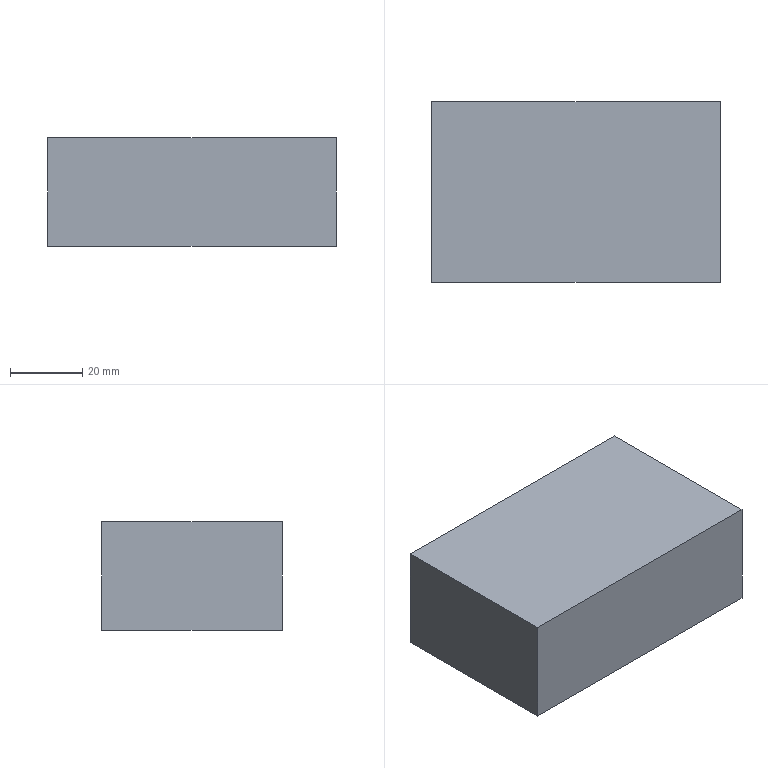Part | NX | features solid 2 | 1 solid | 6 faces | box 80 x 50 x 30 mm | volume 120000 mm3 | plane 6
STEP:
#1=CARTESIAN_POINT('',(41.,-178.,230.));
#2=VERTEX_POINT('',#1);
#3=CARTESIAN_POINT('',(41.,-128.,230.));
#4=VERTEX_POINT('',#3);
#5=CARTESIAN_POINT('',(41.,-467.676,230.));
#6=DIRECTION('',(0.,-1.,0.));
#7=VECTOR('',#6,1000.);
#8=LINE('',#5,#7);
#9=EDGE_CURVE('',#2,#4,#8,.F.);
#10=ORIENTED_EDGE('',*,*,#9,.T.);
#11=CARTESIAN_POINT('',(-39.,-128.,230.));
#12=VERTEX_POINT('',#11);
#13=CARTESIAN_POINT('',(-1894.,-128.,230.));
#14=DIRECTION('',(-1.,0.,0.));
#15=VECTOR('',#14,1000.);
#16=LINE('',#13,#15);
#17=EDGE_CURVE('',#12,#4,#16,.F.);
#18=ORIENTED_EDGE('',*,*,#17,.F.);
#19=CARTESIAN_POINT('',(-39.,-178.,230.));
#20=VERTEX_POINT('',#19);
#21=CARTESIAN_POINT('',(-39.,-178.,230.));
#22=DIRECTION('',(0.,1.,0.));
#23=VECTOR('',#22,1000.);
#24=LINE('',#21,#23);
#25=EDGE_CURVE('',#20,#12,#24,.T.);
#26=ORIENTED_EDGE('',*,*,#25,.F.);
#27=CARTESIAN_POINT('',(-1894.,-178.,230.));
#28=DIRECTION('',(1.,0.,0.));
#29=VECTOR('',#28,1000.);
#30=LINE('',#27,#29);
#31=EDGE_CURVE('',#20,#2,#30,.T.);
#32=ORIENTED_EDGE('',*,*,#31,.T.);
#33=EDGE_LOOP('',(#10,#18,#26,#32));
#34=FACE_BOUND('',#33,.T.);
#35=CARTESIAN_POINT('',(-1894.,-467.676,230.));
#36=DIRECTION('',(0.,0.,-1.));
#37=DIRECTION('',(0.,1.,0.));
#38=AXIS2_PLACEMENT_3D('',#35,#36,#37);
#39=PLANE('',#38);
#40=ADVANCED_FACE('',(#34),#39,.F.);
#41=ORIENTED_EDGE('',*,*,#25,.T.);
#42=CARTESIAN_POINT('',(-39.,-128.,200.));
#43=VERTEX_POINT('',#42);
#44=CARTESIAN_POINT('',(-39.,-128.,10.));
#45=DIRECTION('',(0.,0.,1.));
#46=VECTOR('',#45,1000.);
#47=LINE('',#44,#46);
#48=EDGE_CURVE('',#12,#43,#47,.F.);
#49=ORIENTED_EDGE('',*,*,#48,.T.);
#50=CARTESIAN_POINT('',(-39.,-178.,200.));
#51=VERTEX_POINT('',#50);
#52=CARTESIAN_POINT('',(-39.,-178.,200.));
#53=DIRECTION('',(0.,-1.,0.));
#54=VECTOR('',#53,1000.);
#55=LINE('',#52,#54);
#56=EDGE_CURVE('',#51,#43,#55,.F.);
#57=ORIENTED_EDGE('',*,*,#56,.F.);
#58=CARTESIAN_POINT('',(-39.,-178.,210.));
#59=DIRECTION('',(0.,0.,-1.));
#60=VECTOR('',#59,1000.);
#61=LINE('',#58,#60);
#62=EDGE_CURVE('',#20,#51,#61,.T.);
#63=ORIENTED_EDGE('',*,*,#62,.F.);
#64=EDGE_LOOP('',(#41,#49,#57,#63));
#65=FACE_BOUND('',#64,.T.);
#66=CARTESIAN_POINT('',(-39.,-178.,210.));
#67=DIRECTION('',(1.,0.,0.));
#68=DIRECTION('',(0.,0.,-1.));
#69=AXIS2_PLACEMENT_3D('',#66,#67,#68);
#70=PLANE('',#69);
#71=ADVANCED_FACE('',(#65),#70,.F.);
#72=ORIENTED_EDGE('',*,*,#56,.T.);
#73=CARTESIAN_POINT('',(41.,-128.,200.));
#74=VERTEX_POINT('',#73);
#75=CARTESIAN_POINT('',(-119.,-128.,200.));
#76=DIRECTION('',(-1.,0.,0.));
#77=VECTOR('',#76,1000.);
#78=LINE('',#75,#77);
#79=EDGE_CURVE('',#43,#74,#78,.F.);
#80=ORIENTED_EDGE('',*,*,#79,.T.);
#81=CARTESIAN_POINT('',(41.,-178.,200.));
#82=VERTEX_POINT('',#81);
#83=CARTESIAN_POINT('',(41.,-178.,200.));
#84=DIRECTION('',(0.,-1.,0.));
#85=VECTOR('',#84,1000.);
#86=LINE('',#83,#85);
#87=EDGE_CURVE('',#82,#74,#86,.F.);
#88=ORIENTED_EDGE('',*,*,#87,.F.);
#89=CARTESIAN_POINT('',(-39.,-178.,200.));
#90=DIRECTION('',(1.,0.,0.));
#91=VECTOR('',#90,1000.);
#92=LINE('',#89,#91);
#93=EDGE_CURVE('',#51,#82,#92,.T.);
#94=ORIENTED_EDGE('',*,*,#93,.F.);
#95=EDGE_LOOP('',(#72,#80,#88,#94));
#96=FACE_BOUND('',#95,.T.);
#97=CARTESIAN_POINT('',(-39.,-178.,200.));
#98=DIRECTION('',(0.,0.,1.));
#99=DIRECTION('',(1.,0.,0.));
#100=AXIS2_PLACEMENT_3D('',#97,#98,#99);
#101=PLANE('',#100);
#102=ADVANCED_FACE('',(#96),#101,.F.);
#103=CARTESIAN_POINT('',(41.,-178.,210.));
#104=DIRECTION('',(0.,0.,-1.));
#105=VECTOR('',#104,1000.);
#106=LINE('',#103,#105);
#107=EDGE_CURVE('',#2,#82,#106,.T.);
#108=ORIENTED_EDGE('',*,*,#107,.T.);
#109=ORIENTED_EDGE('',*,*,#87,.T.);
#110=CARTESIAN_POINT('',(41.,-128.,210.));
#111=DIRECTION('',(0.,0.,-1.));
#112=VECTOR('',#111,1000.);
#113=LINE('',#110,#112);
#114=EDGE_CURVE('',#4,#74,#113,.T.);
#115=ORIENTED_EDGE('',*,*,#114,.F.);
#116=ORIENTED_EDGE('',*,*,#9,.F.);
#117=EDGE_LOOP('',(#108,#109,#115,#116));
#118=FACE_BOUND('',#117,.T.);
#119=CARTESIAN_POINT('',(41.,-178.,210.));
#120=DIRECTION('',(1.,0.,0.));
#121=DIRECTION('',(0.,0.,-1.));
#122=AXIS2_PLACEMENT_3D('',#119,#120,#121);
#123=PLANE('',#122);
#124=ADVANCED_FACE('',(#118),#123,.T.);
#125=ORIENTED_EDGE('',*,*,#79,.F.);
#126=ORIENTED_EDGE('',*,*,#48,.F.);
#127=ORIENTED_EDGE('',*,*,#17,.T.);
#128=ORIENTED_EDGE('',*,*,#114,.T.);
#129=EDGE_LOOP('',(#125,#126,#127,#128));
#130=FACE_BOUND('',#129,.T.);
#131=CARTESIAN_POINT('',(-119.,-128.,10.));
#132=DIRECTION('',(0.,-1.,0.));
#133=DIRECTION('',(0.,0.,1.));
#134=AXIS2_PLACEMENT_3D('',#131,#132,#133);
#135=PLANE('',#134);
#136=ADVANCED_FACE('',(#130),#135,.F.);
#137=ORIENTED_EDGE('',*,*,#93,.T.);
#138=ORIENTED_EDGE('',*,*,#107,.F.);
#139=ORIENTED_EDGE('',*,*,#31,.F.);
#140=ORIENTED_EDGE('',*,*,#62,.T.);
#141=EDGE_LOOP('',(#137,#138,#139,#140));
#142=FACE_BOUND('',#141,.T.);
#143=CARTESIAN_POINT('',(-39.,-178.,210.));
#144=DIRECTION('',(0.,1.,0.));
#145=DIRECTION('',(0.,0.,-1.));
#146=AXIS2_PLACEMENT_3D('',#143,#144,#145);
#147=PLANE('',#146);
#148=ADVANCED_FACE('',(#142),#147,.F.);
#149=CLOSED_SHELL('',(#40,#71,#102,#124,#136,#148));
#150=MANIFOLD_SOLID_BREP('',#149);
#151=(LENGTH_UNIT()NAMED_UNIT(*)SI_UNIT(.MILLI.,.METRE.));
#152=UNCERTAINTY_MEASURE_WITH_UNIT(LENGTH_MEASURE(0.00001),#151,'','');
#153=(NAMED_UNIT(*)PLANE_ANGLE_UNIT()SI_UNIT($,.RADIAN.));
#154=(NAMED_UNIT(*)SI_UNIT($,.STERADIAN.)SOLID_ANGLE_UNIT());
#155=(GEOMETRIC_REPRESENTATION_CONTEXT(3)GLOBAL_UNCERTAINTY_ASSIGNED_CONTEXT((#152))GLOBAL_UNIT_ASSIGNED_CONTEXT((#151,#153,#154))REPRESENTATION_CONTEXT('',''));
#156=ADVANCED_BREP_SHAPE_REPRESENTATION('',(#150),#155);